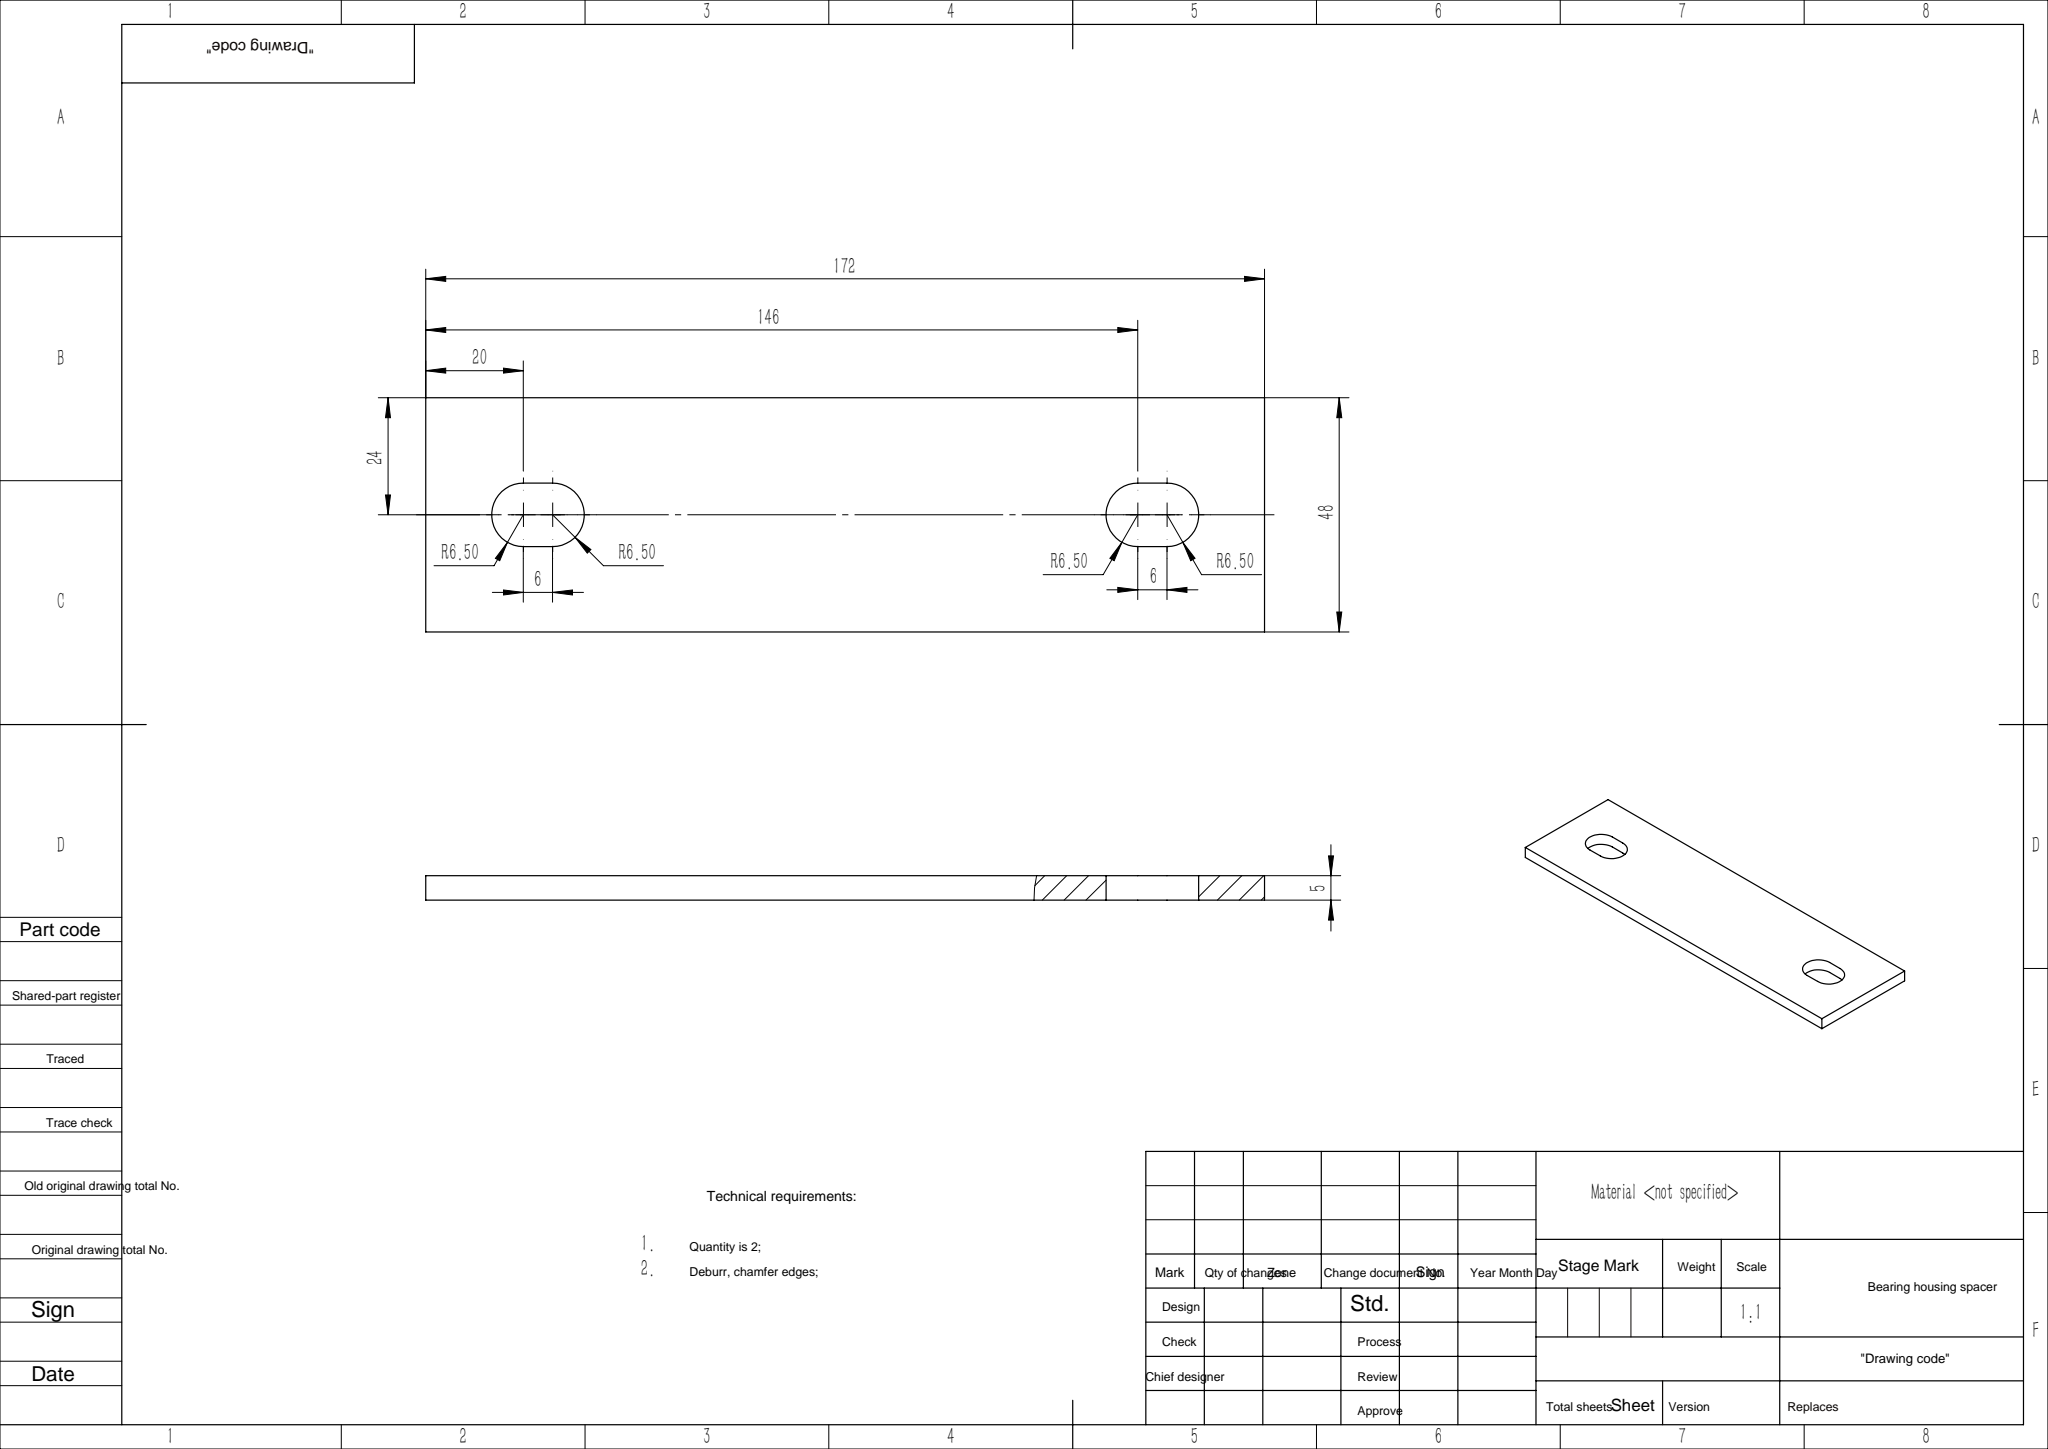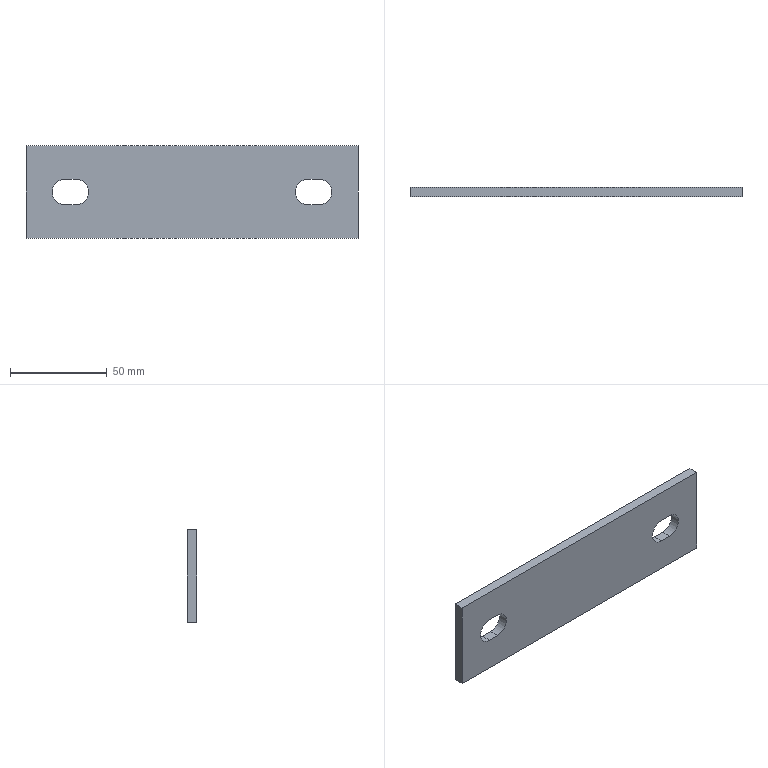Part | SolidWorks | features Cut 1, Extrusion 1 | 1 solid | 14 faces | box 172 x 5 x 48 mm | volume 39173 mm3 | plane 10 | cylinder 4 | commonest cylinder face diameters 13 x4
STEP:
#1=CARTESIAN_POINT('',(86.,0.,24.));
#2=VERTEX_POINT('',#1);
#3=CARTESIAN_POINT('',(86.,0.,-24.));
#4=VERTEX_POINT('',#3);
#5=CARTESIAN_POINT('',(86.,0.,24.));
#6=DIRECTION('',(0.,0.,-1.));
#7=VECTOR('',#6,1000.);
#8=LINE('',#5,#7);
#9=EDGE_CURVE('',#2,#4,#8,.T.);
#10=ORIENTED_EDGE('',*,*,#9,.T.);
#11=CARTESIAN_POINT('',(86.,5.,-24.));
#12=VERTEX_POINT('',#11);
#13=CARTESIAN_POINT('',(86.,5.,-24.));
#14=DIRECTION('',(0.,-1.,0.));
#15=VECTOR('',#14,1000.);
#16=LINE('',#13,#15);
#17=EDGE_CURVE('',#12,#4,#16,.T.);
#18=ORIENTED_EDGE('',*,*,#17,.F.);
#19=CARTESIAN_POINT('',(86.,5.,24.));
#20=VERTEX_POINT('',#19);
#21=CARTESIAN_POINT('',(86.,5.,24.));
#22=DIRECTION('',(0.,0.,-1.));
#23=VECTOR('',#22,1000.);
#24=LINE('',#21,#23);
#25=EDGE_CURVE('',#20,#12,#24,.T.);
#26=ORIENTED_EDGE('',*,*,#25,.F.);
#27=CARTESIAN_POINT('',(86.,5.,24.));
#28=DIRECTION('',(0.,-1.,0.));
#29=VECTOR('',#28,1000.);
#30=LINE('',#27,#29);
#31=EDGE_CURVE('',#20,#2,#30,.T.);
#32=ORIENTED_EDGE('',*,*,#31,.T.);
#33=EDGE_LOOP('',(#10,#18,#26,#32));
#34=FACE_OUTER_BOUND('',#33,.T.);
#35=CARTESIAN_POINT('',(86.,5.,24.));
#36=DIRECTION('',(-1.,0.,0.));
#37=DIRECTION('',(0.,0.,1.));
#38=AXIS2_PLACEMENT_3D('',#35,#36,#37);
#39=PLANE('',#38);
#40=ADVANCED_FACE('',(#34),#39,.F.);
#41=CARTESIAN_POINT('',(-86.,0.,-24.));
#42=VERTEX_POINT('',#41);
#43=CARTESIAN_POINT('',(-86.,0.,-24.));
#44=DIRECTION('',(-1.,0.,0.));
#45=VECTOR('',#44,1000.);
#46=LINE('',#43,#45);
#47=EDGE_CURVE('',#4,#42,#46,.T.);
#48=ORIENTED_EDGE('',*,*,#47,.T.);
#49=CARTESIAN_POINT('',(-86.,5.,-24.));
#50=VERTEX_POINT('',#49);
#51=CARTESIAN_POINT('',(-86.,5.,-24.));
#52=DIRECTION('',(0.,-1.,0.));
#53=VECTOR('',#52,1000.);
#54=LINE('',#51,#53);
#55=EDGE_CURVE('',#50,#42,#54,.T.);
#56=ORIENTED_EDGE('',*,*,#55,.F.);
#57=CARTESIAN_POINT('',(-86.,5.,-24.));
#58=DIRECTION('',(-1.,0.,0.));
#59=VECTOR('',#58,1000.);
#60=LINE('',#57,#59);
#61=EDGE_CURVE('',#12,#50,#60,.T.);
#62=ORIENTED_EDGE('',*,*,#61,.F.);
#63=ORIENTED_EDGE('',*,*,#17,.T.);
#64=EDGE_LOOP('',(#48,#56,#62,#63));
#65=FACE_OUTER_BOUND('',#64,.T.);
#66=CARTESIAN_POINT('',(-86.,5.,-24.));
#67=DIRECTION('',(0.,0.,1.));
#68=DIRECTION('',(1.,0.,0.));
#69=AXIS2_PLACEMENT_3D('',#66,#67,#68);
#70=PLANE('',#69);
#71=ADVANCED_FACE('',(#65),#70,.F.);
#72=CARTESIAN_POINT('',(-86.,0.,24.));
#73=VERTEX_POINT('',#72);
#74=CARTESIAN_POINT('',(-86.,0.,24.));
#75=DIRECTION('',(0.,0.,1.));
#76=VECTOR('',#75,1000.);
#77=LINE('',#74,#76);
#78=EDGE_CURVE('',#42,#73,#77,.T.);
#79=ORIENTED_EDGE('',*,*,#78,.T.);
#80=CARTESIAN_POINT('',(-86.,5.,24.));
#81=VERTEX_POINT('',#80);
#82=CARTESIAN_POINT('',(-86.,5.,24.));
#83=DIRECTION('',(0.,-1.,0.));
#84=VECTOR('',#83,1000.);
#85=LINE('',#82,#84);
#86=EDGE_CURVE('',#81,#73,#85,.T.);
#87=ORIENTED_EDGE('',*,*,#86,.F.);
#88=CARTESIAN_POINT('',(-86.,5.,24.));
#89=DIRECTION('',(0.,0.,1.));
#90=VECTOR('',#89,1000.);
#91=LINE('',#88,#90);
#92=EDGE_CURVE('',#50,#81,#91,.T.);
#93=ORIENTED_EDGE('',*,*,#92,.F.);
#94=ORIENTED_EDGE('',*,*,#55,.T.);
#95=EDGE_LOOP('',(#79,#87,#93,#94));
#96=FACE_OUTER_BOUND('',#95,.T.);
#97=CARTESIAN_POINT('',(-86.,5.,24.));
#98=DIRECTION('',(1.,0.,0.));
#99=DIRECTION('',(0.,0.,-1.));
#100=AXIS2_PLACEMENT_3D('',#97,#98,#99);
#101=PLANE('',#100);
#102=ADVANCED_FACE('',(#96),#101,.F.);
#103=CARTESIAN_POINT('',(-86.,0.,24.));
#104=DIRECTION('',(1.,0.,0.));
#105=VECTOR('',#104,1000.);
#106=LINE('',#103,#105);
#107=EDGE_CURVE('',#73,#2,#106,.T.);
#108=ORIENTED_EDGE('',*,*,#107,.T.);
#109=ORIENTED_EDGE('',*,*,#31,.F.);
#110=CARTESIAN_POINT('',(-86.,5.,24.));
#111=DIRECTION('',(1.,0.,0.));
#112=VECTOR('',#111,1000.);
#113=LINE('',#110,#112);
#114=EDGE_CURVE('',#81,#20,#113,.T.);
#115=ORIENTED_EDGE('',*,*,#114,.F.);
#116=ORIENTED_EDGE('',*,*,#86,.T.);
#117=EDGE_LOOP('',(#108,#109,#115,#116));
#118=FACE_OUTER_BOUND('',#117,.T.);
#119=CARTESIAN_POINT('',(-86.,5.,24.));
#120=DIRECTION('',(0.,0.,-1.));
#121=DIRECTION('',(-1.,0.,0.));
#122=AXIS2_PLACEMENT_3D('',#119,#120,#121);
#123=PLANE('',#122);
#124=ADVANCED_FACE('',(#118),#123,.F.);
#125=CARTESIAN_POINT('',(-60.,5.,-6.5));
#126=VERTEX_POINT('',#125);
#127=CARTESIAN_POINT('',(-66.,5.,-6.5));
#128=VERTEX_POINT('',#127);
#129=CARTESIAN_POINT('',(-66.,5.,-6.5));
#130=DIRECTION('',(-1.,0.,0.));
#131=VECTOR('',#130,1000.);
#132=LINE('',#129,#131);
#133=EDGE_CURVE('',#126,#128,#132,.T.);
#134=ORIENTED_EDGE('',*,*,#133,.F.);
#135=CARTESIAN_POINT('',(-60.,5.,6.5));
#136=VERTEX_POINT('',#135);
#137=CARTESIAN_POINT('',(-60.,5.,0.));
#138=DIRECTION('',(0.,1.,0.));
#139=DIRECTION('',(0.,0.,1.));
#140=AXIS2_PLACEMENT_3D('',#137,#138,#139);
#141=CIRCLE('',#140,6.5);
#142=EDGE_CURVE('',#136,#126,#141,.T.);
#143=ORIENTED_EDGE('',*,*,#142,.F.);
#144=CARTESIAN_POINT('',(-66.,5.,6.5));
#145=VERTEX_POINT('',#144);
#146=CARTESIAN_POINT('',(-60.,5.,6.5));
#147=DIRECTION('',(1.,0.,0.));
#148=VECTOR('',#147,1000.);
#149=LINE('',#146,#148);
#150=EDGE_CURVE('',#145,#136,#149,.T.);
#151=ORIENTED_EDGE('',*,*,#150,.F.);
#152=CARTESIAN_POINT('',(-66.,5.,0.));
#153=DIRECTION('',(0.,1.,0.));
#154=DIRECTION('',(0.,0.,1.));
#155=AXIS2_PLACEMENT_3D('',#152,#153,#154);
#156=CIRCLE('',#155,6.5);
#157=EDGE_CURVE('',#128,#145,#156,.T.);
#158=ORIENTED_EDGE('',*,*,#157,.F.);
#159=EDGE_LOOP('',(#134,#143,#151,#158));
#160=FACE_BOUND('',#159,.T.);
#161=CARTESIAN_POINT('',(66.,5.,-6.5));
#162=VERTEX_POINT('',#161);
#163=CARTESIAN_POINT('',(60.,5.,-6.5));
#164=VERTEX_POINT('',#163);
#165=CARTESIAN_POINT('',(60.,5.,-6.5));
#166=DIRECTION('',(-1.,0.,0.));
#167=VECTOR('',#166,1000.);
#168=LINE('',#165,#167);
#169=EDGE_CURVE('',#162,#164,#168,.T.);
#170=ORIENTED_EDGE('',*,*,#169,.F.);
#171=CARTESIAN_POINT('',(66.,5.,6.5));
#172=VERTEX_POINT('',#171);
#173=CARTESIAN_POINT('',(66.,5.,0.));
#174=DIRECTION('',(0.,1.,0.));
#175=DIRECTION('',(0.,0.,1.));
#176=AXIS2_PLACEMENT_3D('',#173,#174,#175);
#177=CIRCLE('',#176,6.5);
#178=EDGE_CURVE('',#172,#162,#177,.T.);
#179=ORIENTED_EDGE('',*,*,#178,.F.);
#180=CARTESIAN_POINT('',(60.,5.,6.5));
#181=VERTEX_POINT('',#180);
#182=CARTESIAN_POINT('',(66.,5.,6.5));
#183=DIRECTION('',(1.,0.,0.));
#184=VECTOR('',#183,1000.);
#185=LINE('',#182,#184);
#186=EDGE_CURVE('',#181,#172,#185,.T.);
#187=ORIENTED_EDGE('',*,*,#186,.F.);
#188=CARTESIAN_POINT('',(60.,5.,0.));
#189=DIRECTION('',(0.,1.,0.));
#190=DIRECTION('',(0.,0.,1.));
#191=AXIS2_PLACEMENT_3D('',#188,#189,#190);
#192=CIRCLE('',#191,6.5);
#193=EDGE_CURVE('',#164,#181,#192,.T.);
#194=ORIENTED_EDGE('',*,*,#193,.F.);
#195=EDGE_LOOP('',(#170,#179,#187,#194));
#196=FACE_BOUND('',#195,.T.);
#197=ORIENTED_EDGE('',*,*,#25,.T.);
#198=ORIENTED_EDGE('',*,*,#61,.T.);
#199=ORIENTED_EDGE('',*,*,#92,.T.);
#200=ORIENTED_EDGE('',*,*,#114,.T.);
#201=EDGE_LOOP('',(#197,#198,#199,#200));
#202=FACE_OUTER_BOUND('',#201,.T.);
#203=CARTESIAN_POINT('',(0.,5.,0.));
#204=DIRECTION('',(0.,-1.,0.));
#205=DIRECTION('',(0.,0.,-1.));
#206=AXIS2_PLACEMENT_3D('',#203,#204,#205);
#207=PLANE('',#206);
#208=ADVANCED_FACE('',(#160,#196,#202),#207,.F.);
#209=CARTESIAN_POINT('',(-60.,0.,6.5));
#210=VERTEX_POINT('',#209);
#211=CARTESIAN_POINT('',(-60.,0.,-6.5));
#212=VERTEX_POINT('',#211);
#213=CARTESIAN_POINT('',(-60.,0.,0.));
#214=DIRECTION('',(0.,1.,0.));
#215=DIRECTION('',(0.,0.,1.));
#216=AXIS2_PLACEMENT_3D('',#213,#214,#215);
#217=CIRCLE('',#216,6.5);
#218=EDGE_CURVE('',#210,#212,#217,.T.);
#219=ORIENTED_EDGE('',*,*,#218,.T.);
#220=CARTESIAN_POINT('',(-66.,0.,-6.5));
#221=VERTEX_POINT('',#220);
#222=CARTESIAN_POINT('',(-66.,0.,-6.5));
#223=DIRECTION('',(-1.,0.,0.));
#224=VECTOR('',#223,1000.);
#225=LINE('',#222,#224);
#226=EDGE_CURVE('',#212,#221,#225,.T.);
#227=ORIENTED_EDGE('',*,*,#226,.T.);
#228=CARTESIAN_POINT('',(-66.,0.,6.5));
#229=VERTEX_POINT('',#228);
#230=CARTESIAN_POINT('',(-66.,0.,0.));
#231=DIRECTION('',(0.,1.,0.));
#232=DIRECTION('',(0.,0.,1.));
#233=AXIS2_PLACEMENT_3D('',#230,#231,#232);
#234=CIRCLE('',#233,6.5);
#235=EDGE_CURVE('',#221,#229,#234,.T.);
#236=ORIENTED_EDGE('',*,*,#235,.T.);
#237=CARTESIAN_POINT('',(-60.,0.,6.5));
#238=DIRECTION('',(1.,0.,0.));
#239=VECTOR('',#238,1000.);
#240=LINE('',#237,#239);
#241=EDGE_CURVE('',#229,#210,#240,.T.);
#242=ORIENTED_EDGE('',*,*,#241,.T.);
#243=EDGE_LOOP('',(#219,#227,#236,#242));
#244=FACE_BOUND('',#243,.T.);
#245=CARTESIAN_POINT('',(66.,0.,6.5));
#246=VERTEX_POINT('',#245);
#247=CARTESIAN_POINT('',(66.,0.,-6.5));
#248=VERTEX_POINT('',#247);
#249=CARTESIAN_POINT('',(66.,0.,0.));
#250=DIRECTION('',(0.,1.,0.));
#251=DIRECTION('',(0.,0.,1.));
#252=AXIS2_PLACEMENT_3D('',#249,#250,#251);
#253=CIRCLE('',#252,6.5);
#254=EDGE_CURVE('',#246,#248,#253,.T.);
#255=ORIENTED_EDGE('',*,*,#254,.T.);
#256=CARTESIAN_POINT('',(60.,0.,-6.5));
#257=VERTEX_POINT('',#256);
#258=CARTESIAN_POINT('',(60.,0.,-6.5));
#259=DIRECTION('',(-1.,0.,0.));
#260=VECTOR('',#259,1000.);
#261=LINE('',#258,#260);
#262=EDGE_CURVE('',#248,#257,#261,.T.);
#263=ORIENTED_EDGE('',*,*,#262,.T.);
#264=CARTESIAN_POINT('',(60.,0.,6.5));
#265=VERTEX_POINT('',#264);
#266=CARTESIAN_POINT('',(60.,0.,0.));
#267=DIRECTION('',(0.,1.,0.));
#268=DIRECTION('',(0.,0.,1.));
#269=AXIS2_PLACEMENT_3D('',#266,#267,#268);
#270=CIRCLE('',#269,6.5);
#271=EDGE_CURVE('',#257,#265,#270,.T.);
#272=ORIENTED_EDGE('',*,*,#271,.T.);
#273=CARTESIAN_POINT('',(66.,0.,6.5));
#274=DIRECTION('',(1.,0.,0.));
#275=VECTOR('',#274,1000.);
#276=LINE('',#273,#275);
#277=EDGE_CURVE('',#265,#246,#276,.T.);
#278=ORIENTED_EDGE('',*,*,#277,.T.);
#279=EDGE_LOOP('',(#255,#263,#272,#278));
#280=FACE_BOUND('',#279,.T.);
#281=ORIENTED_EDGE('',*,*,#9,.F.);
#282=ORIENTED_EDGE('',*,*,#107,.F.);
#283=ORIENTED_EDGE('',*,*,#78,.F.);
#284=ORIENTED_EDGE('',*,*,#47,.F.);
#285=EDGE_LOOP('',(#281,#282,#283,#284));
#286=FACE_OUTER_BOUND('',#285,.T.);
#287=CARTESIAN_POINT('',(0.,0.,0.));
#288=DIRECTION('',(0.,-1.,0.));
#289=DIRECTION('',(0.,0.,-1.));
#290=AXIS2_PLACEMENT_3D('',#287,#288,#289);
#291=PLANE('',#290);
#292=ADVANCED_FACE('',(#244,#280,#286),#291,.T.);
#293=ORIENTED_EDGE('',*,*,#178,.T.);
#294=CARTESIAN_POINT('',(66.,0.,-6.5));
#295=DIRECTION('',(0.,1.,0.));
#296=VECTOR('',#295,1000.);
#297=LINE('',#294,#296);
#298=EDGE_CURVE('',#248,#162,#297,.T.);
#299=ORIENTED_EDGE('',*,*,#298,.F.);
#300=ORIENTED_EDGE('',*,*,#254,.F.);
#301=CARTESIAN_POINT('',(66.,0.,6.5));
#302=DIRECTION('',(0.,1.,0.));
#303=VECTOR('',#302,1000.);
#304=LINE('',#301,#303);
#305=EDGE_CURVE('',#246,#172,#304,.T.);
#306=ORIENTED_EDGE('',*,*,#305,.T.);
#307=EDGE_LOOP('',(#293,#299,#300,#306));
#308=FACE_OUTER_BOUND('',#307,.T.);
#309=CARTESIAN_POINT('',(66.,0.,0.));
#310=DIRECTION('',(0.,1.,0.));
#311=DIRECTION('',(0.,0.,1.));
#312=AXIS2_PLACEMENT_3D('',#309,#310,#311);
#313=CYLINDRICAL_SURFACE('',#312,6.5);
#314=ADVANCED_FACE('',(#308),#313,.F.);
#315=ORIENTED_EDGE('',*,*,#186,.T.);
#316=ORIENTED_EDGE('',*,*,#305,.F.);
#317=ORIENTED_EDGE('',*,*,#277,.F.);
#318=CARTESIAN_POINT('',(60.,0.,6.5));
#319=DIRECTION('',(0.,1.,0.));
#320=VECTOR('',#319,1000.);
#321=LINE('',#318,#320);
#322=EDGE_CURVE('',#265,#181,#321,.T.);
#323=ORIENTED_EDGE('',*,*,#322,.T.);
#324=EDGE_LOOP('',(#315,#316,#317,#323));
#325=FACE_OUTER_BOUND('',#324,.T.);
#326=CARTESIAN_POINT('',(66.,0.,6.5));
#327=DIRECTION('',(0.,0.,1.));
#328=DIRECTION('',(1.,0.,0.));
#329=AXIS2_PLACEMENT_3D('',#326,#327,#328);
#330=PLANE('',#329);
#331=ADVANCED_FACE('',(#325),#330,.F.);
#332=ORIENTED_EDGE('',*,*,#193,.T.);
#333=ORIENTED_EDGE('',*,*,#322,.F.);
#334=ORIENTED_EDGE('',*,*,#271,.F.);
#335=CARTESIAN_POINT('',(60.,0.,-6.5));
#336=DIRECTION('',(0.,1.,0.));
#337=VECTOR('',#336,1000.);
#338=LINE('',#335,#337);
#339=EDGE_CURVE('',#257,#164,#338,.T.);
#340=ORIENTED_EDGE('',*,*,#339,.T.);
#341=EDGE_LOOP('',(#332,#333,#334,#340));
#342=FACE_OUTER_BOUND('',#341,.T.);
#343=CARTESIAN_POINT('',(60.,0.,0.));
#344=DIRECTION('',(0.,1.,0.));
#345=DIRECTION('',(0.,0.,1.));
#346=AXIS2_PLACEMENT_3D('',#343,#344,#345);
#347=CYLINDRICAL_SURFACE('',#346,6.5);
#348=ADVANCED_FACE('',(#342),#347,.F.);
#349=ORIENTED_EDGE('',*,*,#169,.T.);
#350=ORIENTED_EDGE('',*,*,#339,.F.);
#351=ORIENTED_EDGE('',*,*,#262,.F.);
#352=ORIENTED_EDGE('',*,*,#298,.T.);
#353=EDGE_LOOP('',(#349,#350,#351,#352));
#354=FACE_OUTER_BOUND('',#353,.T.);
#355=CARTESIAN_POINT('',(60.,0.,-6.5));
#356=DIRECTION('',(0.,0.,-1.));
#357=DIRECTION('',(-1.,0.,0.));
#358=AXIS2_PLACEMENT_3D('',#355,#356,#357);
#359=PLANE('',#358);
#360=ADVANCED_FACE('',(#354),#359,.F.);
#361=ORIENTED_EDGE('',*,*,#142,.T.);
#362=CARTESIAN_POINT('',(-60.,0.,-6.5));
#363=DIRECTION('',(0.,1.,0.));
#364=VECTOR('',#363,1000.);
#365=LINE('',#362,#364);
#366=EDGE_CURVE('',#212,#126,#365,.T.);
#367=ORIENTED_EDGE('',*,*,#366,.F.);
#368=ORIENTED_EDGE('',*,*,#218,.F.);
#369=CARTESIAN_POINT('',(-60.,0.,6.5));
#370=DIRECTION('',(0.,1.,0.));
#371=VECTOR('',#370,1000.);
#372=LINE('',#369,#371);
#373=EDGE_CURVE('',#210,#136,#372,.T.);
#374=ORIENTED_EDGE('',*,*,#373,.T.);
#375=EDGE_LOOP('',(#361,#367,#368,#374));
#376=FACE_OUTER_BOUND('',#375,.T.);
#377=CARTESIAN_POINT('',(-60.,0.,0.));
#378=DIRECTION('',(0.,1.,0.));
#379=DIRECTION('',(0.,0.,1.));
#380=AXIS2_PLACEMENT_3D('',#377,#378,#379);
#381=CYLINDRICAL_SURFACE('',#380,6.5);
#382=ADVANCED_FACE('',(#376),#381,.F.);
#383=ORIENTED_EDGE('',*,*,#150,.T.);
#384=ORIENTED_EDGE('',*,*,#373,.F.);
#385=ORIENTED_EDGE('',*,*,#241,.F.);
#386=CARTESIAN_POINT('',(-66.,0.,6.5));
#387=DIRECTION('',(0.,1.,0.));
#388=VECTOR('',#387,1000.);
#389=LINE('',#386,#388);
#390=EDGE_CURVE('',#229,#145,#389,.T.);
#391=ORIENTED_EDGE('',*,*,#390,.T.);
#392=EDGE_LOOP('',(#383,#384,#385,#391));
#393=FACE_OUTER_BOUND('',#392,.T.);
#394=CARTESIAN_POINT('',(-60.,0.,6.5));
#395=DIRECTION('',(0.,0.,1.));
#396=DIRECTION('',(1.,0.,0.));
#397=AXIS2_PLACEMENT_3D('',#394,#395,#396);
#398=PLANE('',#397);
#399=ADVANCED_FACE('',(#393),#398,.F.);
#400=ORIENTED_EDGE('',*,*,#157,.T.);
#401=ORIENTED_EDGE('',*,*,#390,.F.);
#402=ORIENTED_EDGE('',*,*,#235,.F.);
#403=CARTESIAN_POINT('',(-66.,0.,-6.5));
#404=DIRECTION('',(0.,1.,0.));
#405=VECTOR('',#404,1000.);
#406=LINE('',#403,#405);
#407=EDGE_CURVE('',#221,#128,#406,.T.);
#408=ORIENTED_EDGE('',*,*,#407,.T.);
#409=EDGE_LOOP('',(#400,#401,#402,#408));
#410=FACE_OUTER_BOUND('',#409,.T.);
#411=CARTESIAN_POINT('',(-66.,0.,0.));
#412=DIRECTION('',(0.,1.,0.));
#413=DIRECTION('',(0.,0.,1.));
#414=AXIS2_PLACEMENT_3D('',#411,#412,#413);
#415=CYLINDRICAL_SURFACE('',#414,6.5);
#416=ADVANCED_FACE('',(#410),#415,.F.);
#417=ORIENTED_EDGE('',*,*,#133,.T.);
#418=ORIENTED_EDGE('',*,*,#407,.F.);
#419=ORIENTED_EDGE('',*,*,#226,.F.);
#420=ORIENTED_EDGE('',*,*,#366,.T.);
#421=EDGE_LOOP('',(#417,#418,#419,#420));
#422=FACE_OUTER_BOUND('',#421,.T.);
#423=CARTESIAN_POINT('',(-66.,0.,-6.5));
#424=DIRECTION('',(0.,0.,-1.));
#425=DIRECTION('',(-1.,0.,0.));
#426=AXIS2_PLACEMENT_3D('',#423,#424,#425);
#427=PLANE('',#426);
#428=ADVANCED_FACE('',(#422),#427,.F.);
#429=CLOSED_SHELL('',(#40,#71,#102,#124,#208,#292,#314,#331,#348,#360,#382,#399,#416,#428));
#430=MANIFOLD_SOLID_BREP('',#429);
#431=CARTESIAN_POINT('',(0.,0.,0.));
#432=DIRECTION('',(0.,0.,1.));
#433=DIRECTION('',(1.,0.,0.));
#434=AXIS2_PLACEMENT_3D('',#431,#432,#433);
#435=(LENGTH_UNIT()NAMED_UNIT(*)SI_UNIT(.MILLI.,.METRE.));
#436=UNCERTAINTY_MEASURE_WITH_UNIT(LENGTH_MEASURE(0.00001),#435,'','');
#437=(NAMED_UNIT(*)PLANE_ANGLE_UNIT()SI_UNIT($,.RADIAN.));
#438=(NAMED_UNIT(*)SI_UNIT($,.STERADIAN.)SOLID_ANGLE_UNIT());
#439=(GEOMETRIC_REPRESENTATION_CONTEXT(3)GLOBAL_UNCERTAINTY_ASSIGNED_CONTEXT((#436))GLOBAL_UNIT_ASSIGNED_CONTEXT((#435,#437,#438))REPRESENTATION_CONTEXT('',''));
#440=ADVANCED_BREP_SHAPE_REPRESENTATION('',(#430,#434),#439);